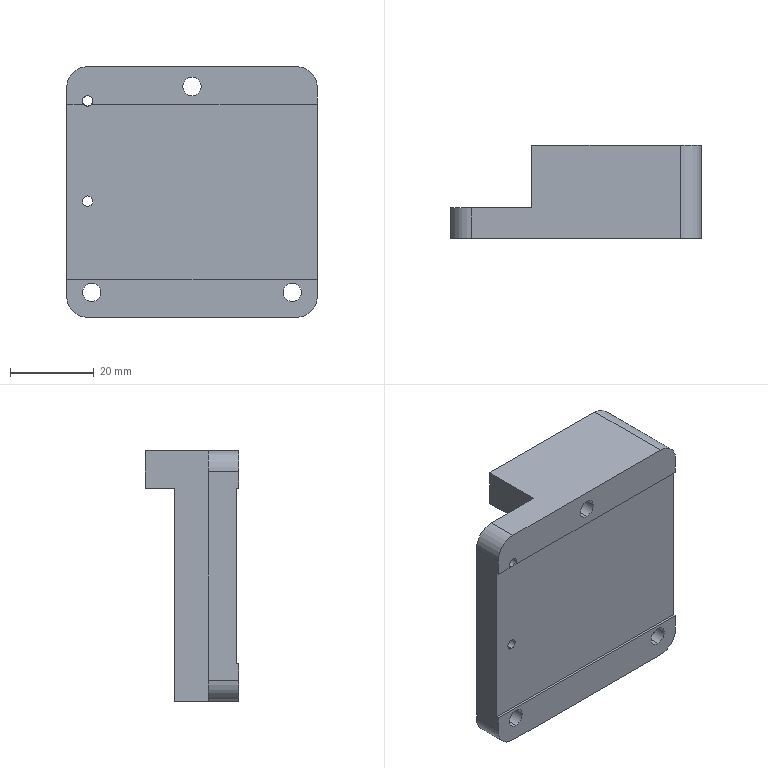Part | SolidWorks | features ICE 5, HoleWzd 2, Extrusion 1, Fillet 1 | 1 solid | 54 faces | box 60 x 22.3 x 60 mm | volume 44842 mm3 | cylinder 28 | plane 18 | cone 8 | commonest cylinder face diameters 2.5 x12 4.4 x6 7.5 x6 10 x4